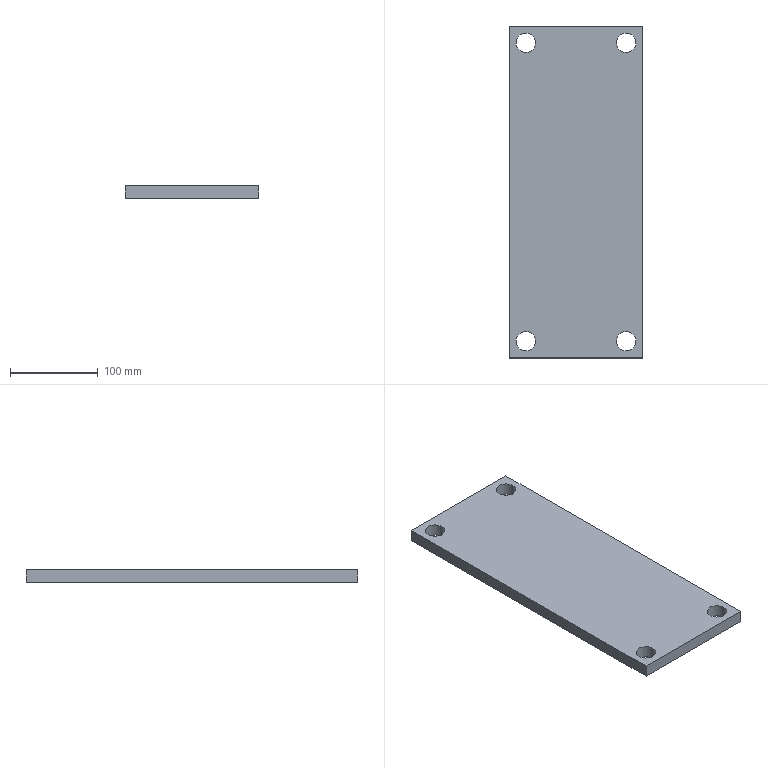Part | SolidWorks | features Extrusion 1 | 1 solid | 14 faces | box 152.4 x 377.95 x 14 mm | volume 784620 mm3 | cylinder 8 | plane 6 | commonest cylinder face diameters 22.25 x8
STEP:
#1=CARTESIAN_POINT('',(-68.275,-169.862,14.));
#2=VERTEX_POINT('',#1);
#3=CARTESIAN_POINT('',(-46.025,-169.862,14.));
#4=VERTEX_POINT('',#3);
#5=CARTESIAN_POINT('',(-57.15,-169.862,14.));
#6=DIRECTION('',(0.,0.,1.));
#7=DIRECTION('',(1.,0.,0.));
#8=AXIS2_PLACEMENT_3D('',#5,#6,#7);
#9=CIRCLE('',#8,11.125);
#10=EDGE_CURVE('',#2,#4,#9,.T.);
#11=ORIENTED_EDGE('',*,*,#10,.T.);
#12=CARTESIAN_POINT('',(-46.025,-169.862,0.));
#13=VERTEX_POINT('',#12);
#14=CARTESIAN_POINT('',(-46.025,-169.862,14.));
#15=DIRECTION('',(0.,0.,-1.));
#16=VECTOR('',#15,1000.);
#17=LINE('',#14,#16);
#18=EDGE_CURVE('',#4,#13,#17,.T.);
#19=ORIENTED_EDGE('',*,*,#18,.T.);
#20=CARTESIAN_POINT('',(-68.275,-169.862,0.));
#21=VERTEX_POINT('',#20);
#22=CARTESIAN_POINT('',(-57.15,-169.862,0.));
#23=DIRECTION('',(0.,0.,1.));
#24=DIRECTION('',(1.,0.,0.));
#25=AXIS2_PLACEMENT_3D('',#22,#23,#24);
#26=CIRCLE('',#25,11.125);
#27=EDGE_CURVE('',#21,#13,#26,.T.);
#28=ORIENTED_EDGE('',*,*,#27,.F.);
#29=CARTESIAN_POINT('',(-68.275,-169.862,14.));
#30=DIRECTION('',(0.,0.,-1.));
#31=VECTOR('',#30,1000.);
#32=LINE('',#29,#31);
#33=EDGE_CURVE('',#2,#21,#32,.T.);
#34=ORIENTED_EDGE('',*,*,#33,.F.);
#35=EDGE_LOOP('',(#11,#19,#28,#34));
#36=FACE_OUTER_BOUND('',#35,.T.);
#37=CARTESIAN_POINT('',(-57.15,-169.862,14.));
#38=DIRECTION('',(0.,0.,-1.));
#39=DIRECTION('',(-1.,0.,0.));
#40=AXIS2_PLACEMENT_3D('',#37,#38,#39);
#41=CYLINDRICAL_SURFACE('',#40,11.125);
#42=ADVANCED_FACE('',(#36),#41,.F.);
#43=CARTESIAN_POINT('',(46.025,-169.862,14.));
#44=VERTEX_POINT('',#43);
#45=CARTESIAN_POINT('',(68.275,-169.862,14.));
#46=VERTEX_POINT('',#45);
#47=CARTESIAN_POINT('',(57.15,-169.862,14.));
#48=DIRECTION('',(0.,0.,1.));
#49=DIRECTION('',(1.,0.,0.));
#50=AXIS2_PLACEMENT_3D('',#47,#48,#49);
#51=CIRCLE('',#50,11.125);
#52=EDGE_CURVE('',#44,#46,#51,.T.);
#53=ORIENTED_EDGE('',*,*,#52,.T.);
#54=CARTESIAN_POINT('',(68.275,-169.862,0.));
#55=VERTEX_POINT('',#54);
#56=CARTESIAN_POINT('',(68.275,-169.862,14.));
#57=DIRECTION('',(0.,0.,-1.));
#58=VECTOR('',#57,1000.);
#59=LINE('',#56,#58);
#60=EDGE_CURVE('',#46,#55,#59,.T.);
#61=ORIENTED_EDGE('',*,*,#60,.T.);
#62=CARTESIAN_POINT('',(46.025,-169.862,0.));
#63=VERTEX_POINT('',#62);
#64=CARTESIAN_POINT('',(57.15,-169.862,0.));
#65=DIRECTION('',(0.,0.,1.));
#66=DIRECTION('',(1.,0.,0.));
#67=AXIS2_PLACEMENT_3D('',#64,#65,#66);
#68=CIRCLE('',#67,11.125);
#69=EDGE_CURVE('',#63,#55,#68,.T.);
#70=ORIENTED_EDGE('',*,*,#69,.F.);
#71=CARTESIAN_POINT('',(46.025,-169.862,14.));
#72=DIRECTION('',(0.,0.,-1.));
#73=VECTOR('',#72,1000.);
#74=LINE('',#71,#73);
#75=EDGE_CURVE('',#44,#63,#74,.T.);
#76=ORIENTED_EDGE('',*,*,#75,.F.);
#77=EDGE_LOOP('',(#53,#61,#70,#76));
#78=FACE_OUTER_BOUND('',#77,.T.);
#79=CARTESIAN_POINT('',(57.15,-169.862,14.));
#80=DIRECTION('',(0.,0.,-1.));
#81=DIRECTION('',(-1.,0.,0.));
#82=AXIS2_PLACEMENT_3D('',#79,#80,#81);
#83=CYLINDRICAL_SURFACE('',#82,11.125);
#84=ADVANCED_FACE('',(#78),#83,.F.);
#85=CARTESIAN_POINT('',(46.025,169.863,14.));
#86=VERTEX_POINT('',#85);
#87=CARTESIAN_POINT('',(68.275,169.863,14.));
#88=VERTEX_POINT('',#87);
#89=CARTESIAN_POINT('',(57.15,169.863,14.));
#90=DIRECTION('',(0.,0.,1.));
#91=DIRECTION('',(1.,0.,0.));
#92=AXIS2_PLACEMENT_3D('',#89,#90,#91);
#93=CIRCLE('',#92,11.125);
#94=EDGE_CURVE('',#86,#88,#93,.T.);
#95=ORIENTED_EDGE('',*,*,#94,.T.);
#96=CARTESIAN_POINT('',(68.275,169.863,0.));
#97=VERTEX_POINT('',#96);
#98=CARTESIAN_POINT('',(68.275,169.863,14.));
#99=DIRECTION('',(0.,0.,-1.));
#100=VECTOR('',#99,1000.);
#101=LINE('',#98,#100);
#102=EDGE_CURVE('',#88,#97,#101,.T.);
#103=ORIENTED_EDGE('',*,*,#102,.T.);
#104=CARTESIAN_POINT('',(46.025,169.863,0.));
#105=VERTEX_POINT('',#104);
#106=CARTESIAN_POINT('',(57.15,169.863,0.));
#107=DIRECTION('',(0.,0.,1.));
#108=DIRECTION('',(1.,0.,0.));
#109=AXIS2_PLACEMENT_3D('',#106,#107,#108);
#110=CIRCLE('',#109,11.125);
#111=EDGE_CURVE('',#105,#97,#110,.T.);
#112=ORIENTED_EDGE('',*,*,#111,.F.);
#113=CARTESIAN_POINT('',(46.025,169.863,14.));
#114=DIRECTION('',(0.,0.,-1.));
#115=VECTOR('',#114,1000.);
#116=LINE('',#113,#115);
#117=EDGE_CURVE('',#86,#105,#116,.T.);
#118=ORIENTED_EDGE('',*,*,#117,.F.);
#119=EDGE_LOOP('',(#95,#103,#112,#118));
#120=FACE_OUTER_BOUND('',#119,.T.);
#121=CARTESIAN_POINT('',(57.15,169.863,14.));
#122=DIRECTION('',(0.,0.,-1.));
#123=DIRECTION('',(-1.,0.,0.));
#124=AXIS2_PLACEMENT_3D('',#121,#122,#123);
#125=CYLINDRICAL_SURFACE('',#124,11.125);
#126=ADVANCED_FACE('',(#120),#125,.F.);
#127=CARTESIAN_POINT('',(-68.275,169.863,14.));
#128=VERTEX_POINT('',#127);
#129=CARTESIAN_POINT('',(-46.025,169.863,14.));
#130=VERTEX_POINT('',#129);
#131=CARTESIAN_POINT('',(-57.15,169.863,14.));
#132=DIRECTION('',(0.,0.,1.));
#133=DIRECTION('',(1.,0.,0.));
#134=AXIS2_PLACEMENT_3D('',#131,#132,#133);
#135=CIRCLE('',#134,11.125);
#136=EDGE_CURVE('',#128,#130,#135,.T.);
#137=ORIENTED_EDGE('',*,*,#136,.T.);
#138=CARTESIAN_POINT('',(-46.025,169.863,0.));
#139=VERTEX_POINT('',#138);
#140=CARTESIAN_POINT('',(-46.025,169.863,14.));
#141=DIRECTION('',(0.,0.,-1.));
#142=VECTOR('',#141,1000.);
#143=LINE('',#140,#142);
#144=EDGE_CURVE('',#130,#139,#143,.T.);
#145=ORIENTED_EDGE('',*,*,#144,.T.);
#146=CARTESIAN_POINT('',(-68.275,169.863,0.));
#147=VERTEX_POINT('',#146);
#148=CARTESIAN_POINT('',(-57.15,169.863,0.));
#149=DIRECTION('',(0.,0.,1.));
#150=DIRECTION('',(1.,0.,0.));
#151=AXIS2_PLACEMENT_3D('',#148,#149,#150);
#152=CIRCLE('',#151,11.125);
#153=EDGE_CURVE('',#147,#139,#152,.T.);
#154=ORIENTED_EDGE('',*,*,#153,.F.);
#155=CARTESIAN_POINT('',(-68.275,169.863,14.));
#156=DIRECTION('',(0.,0.,-1.));
#157=VECTOR('',#156,1000.);
#158=LINE('',#155,#157);
#159=EDGE_CURVE('',#128,#147,#158,.T.);
#160=ORIENTED_EDGE('',*,*,#159,.F.);
#161=EDGE_LOOP('',(#137,#145,#154,#160));
#162=FACE_OUTER_BOUND('',#161,.T.);
#163=CARTESIAN_POINT('',(-57.15,169.863,14.));
#164=DIRECTION('',(0.,0.,-1.));
#165=DIRECTION('',(-1.,0.,0.));
#166=AXIS2_PLACEMENT_3D('',#163,#164,#165);
#167=CYLINDRICAL_SURFACE('',#166,11.125);
#168=ADVANCED_FACE('',(#162),#167,.F.);
#169=ORIENTED_EDGE('',*,*,#52,.F.);
#170=CARTESIAN_POINT('',(57.15,-169.862,14.));
#171=DIRECTION('',(0.,0.,1.));
#172=DIRECTION('',(1.,0.,0.));
#173=AXIS2_PLACEMENT_3D('',#170,#171,#172);
#174=CIRCLE('',#173,11.125);
#175=EDGE_CURVE('',#46,#44,#174,.T.);
#176=ORIENTED_EDGE('',*,*,#175,.F.);
#177=EDGE_LOOP('',(#169,#176));
#178=FACE_BOUND('',#177,.T.);
#179=ORIENTED_EDGE('',*,*,#136,.F.);
#180=CARTESIAN_POINT('',(-57.15,169.863,14.));
#181=DIRECTION('',(0.,0.,1.));
#182=DIRECTION('',(1.,0.,0.));
#183=AXIS2_PLACEMENT_3D('',#180,#181,#182);
#184=CIRCLE('',#183,11.125);
#185=EDGE_CURVE('',#130,#128,#184,.T.);
#186=ORIENTED_EDGE('',*,*,#185,.F.);
#187=EDGE_LOOP('',(#179,#186));
#188=FACE_BOUND('',#187,.T.);
#189=CARTESIAN_POINT('',(76.2,-188.975,14.));
#190=VERTEX_POINT('',#189);
#191=CARTESIAN_POINT('',(76.2,188.975,14.));
#192=VERTEX_POINT('',#191);
#193=CARTESIAN_POINT('',(76.2,188.975,14.));
#194=DIRECTION('',(0.,1.,0.));
#195=VECTOR('',#194,1000.);
#196=LINE('',#193,#195);
#197=EDGE_CURVE('',#190,#192,#196,.T.);
#198=ORIENTED_EDGE('',*,*,#197,.T.);
#199=CARTESIAN_POINT('',(-76.2,188.975,14.));
#200=VERTEX_POINT('',#199);
#201=CARTESIAN_POINT('',(-76.2,188.975,14.));
#202=DIRECTION('',(-1.,0.,0.));
#203=VECTOR('',#202,1000.);
#204=LINE('',#201,#203);
#205=EDGE_CURVE('',#192,#200,#204,.T.);
#206=ORIENTED_EDGE('',*,*,#205,.T.);
#207=CARTESIAN_POINT('',(-76.2,-188.975,14.));
#208=VERTEX_POINT('',#207);
#209=CARTESIAN_POINT('',(-76.2,188.975,14.));
#210=DIRECTION('',(0.,-1.,0.));
#211=VECTOR('',#210,1000.);
#212=LINE('',#209,#211);
#213=EDGE_CURVE('',#200,#208,#212,.T.);
#214=ORIENTED_EDGE('',*,*,#213,.T.);
#215=CARTESIAN_POINT('',(-76.2,-188.975,14.));
#216=DIRECTION('',(1.,0.,0.));
#217=VECTOR('',#216,1000.);
#218=LINE('',#215,#217);
#219=EDGE_CURVE('',#208,#190,#218,.T.);
#220=ORIENTED_EDGE('',*,*,#219,.T.);
#221=EDGE_LOOP('',(#198,#206,#214,#220));
#222=FACE_OUTER_BOUND('',#221,.T.);
#223=ORIENTED_EDGE('',*,*,#94,.F.);
#224=CARTESIAN_POINT('',(57.15,169.863,14.));
#225=DIRECTION('',(0.,0.,1.));
#226=DIRECTION('',(1.,0.,0.));
#227=AXIS2_PLACEMENT_3D('',#224,#225,#226);
#228=CIRCLE('',#227,11.125);
#229=EDGE_CURVE('',#88,#86,#228,.T.);
#230=ORIENTED_EDGE('',*,*,#229,.F.);
#231=EDGE_LOOP('',(#223,#230));
#232=FACE_BOUND('',#231,.T.);
#233=ORIENTED_EDGE('',*,*,#10,.F.);
#234=CARTESIAN_POINT('',(-57.15,-169.862,14.));
#235=DIRECTION('',(0.,0.,1.));
#236=DIRECTION('',(1.,0.,0.));
#237=AXIS2_PLACEMENT_3D('',#234,#235,#236);
#238=CIRCLE('',#237,11.125);
#239=EDGE_CURVE('',#4,#2,#238,.T.);
#240=ORIENTED_EDGE('',*,*,#239,.F.);
#241=EDGE_LOOP('',(#233,#240));
#242=FACE_BOUND('',#241,.T.);
#243=CARTESIAN_POINT('',(76.2,-188.975,14.));
#244=DIRECTION('',(0.,0.,1.));
#245=DIRECTION('',(1.,0.,0.));
#246=AXIS2_PLACEMENT_3D('',#243,#244,#245);
#247=PLANE('',#246);
#248=ADVANCED_FACE('',(#178,#188,#222,#232,#242),#247,.T.);
#249=ORIENTED_EDGE('',*,*,#69,.T.);
#250=CARTESIAN_POINT('',(57.15,-169.862,0.));
#251=DIRECTION('',(0.,0.,1.));
#252=DIRECTION('',(1.,0.,0.));
#253=AXIS2_PLACEMENT_3D('',#250,#251,#252);
#254=CIRCLE('',#253,11.125);
#255=EDGE_CURVE('',#55,#63,#254,.T.);
#256=ORIENTED_EDGE('',*,*,#255,.T.);
#257=EDGE_LOOP('',(#249,#256));
#258=FACE_BOUND('',#257,.T.);
#259=ORIENTED_EDGE('',*,*,#153,.T.);
#260=CARTESIAN_POINT('',(-57.15,169.863,0.));
#261=DIRECTION('',(0.,0.,1.));
#262=DIRECTION('',(1.,0.,0.));
#263=AXIS2_PLACEMENT_3D('',#260,#261,#262);
#264=CIRCLE('',#263,11.125);
#265=EDGE_CURVE('',#139,#147,#264,.T.);
#266=ORIENTED_EDGE('',*,*,#265,.T.);
#267=EDGE_LOOP('',(#259,#266));
#268=FACE_BOUND('',#267,.T.);
#269=CARTESIAN_POINT('',(76.2,-188.975,0.));
#270=VERTEX_POINT('',#269);
#271=CARTESIAN_POINT('',(76.2,188.975,0.));
#272=VERTEX_POINT('',#271);
#273=CARTESIAN_POINT('',(76.2,188.975,0.));
#274=DIRECTION('',(0.,1.,0.));
#275=VECTOR('',#274,1000.);
#276=LINE('',#273,#275);
#277=EDGE_CURVE('',#270,#272,#276,.T.);
#278=ORIENTED_EDGE('',*,*,#277,.F.);
#279=CARTESIAN_POINT('',(-76.2,-188.975,0.));
#280=VERTEX_POINT('',#279);
#281=CARTESIAN_POINT('',(-76.2,-188.975,0.));
#282=DIRECTION('',(1.,0.,0.));
#283=VECTOR('',#282,1000.);
#284=LINE('',#281,#283);
#285=EDGE_CURVE('',#280,#270,#284,.T.);
#286=ORIENTED_EDGE('',*,*,#285,.F.);
#287=CARTESIAN_POINT('',(-76.2,188.975,0.));
#288=VERTEX_POINT('',#287);
#289=CARTESIAN_POINT('',(-76.2,188.975,0.));
#290=DIRECTION('',(0.,-1.,0.));
#291=VECTOR('',#290,1000.);
#292=LINE('',#289,#291);
#293=EDGE_CURVE('',#288,#280,#292,.T.);
#294=ORIENTED_EDGE('',*,*,#293,.F.);
#295=CARTESIAN_POINT('',(-76.2,188.975,0.));
#296=DIRECTION('',(-1.,0.,0.));
#297=VECTOR('',#296,1000.);
#298=LINE('',#295,#297);
#299=EDGE_CURVE('',#272,#288,#298,.T.);
#300=ORIENTED_EDGE('',*,*,#299,.F.);
#301=EDGE_LOOP('',(#278,#286,#294,#300));
#302=FACE_OUTER_BOUND('',#301,.T.);
#303=ORIENTED_EDGE('',*,*,#111,.T.);
#304=CARTESIAN_POINT('',(57.15,169.863,0.));
#305=DIRECTION('',(0.,0.,1.));
#306=DIRECTION('',(1.,0.,0.));
#307=AXIS2_PLACEMENT_3D('',#304,#305,#306);
#308=CIRCLE('',#307,11.125);
#309=EDGE_CURVE('',#97,#105,#308,.T.);
#310=ORIENTED_EDGE('',*,*,#309,.T.);
#311=EDGE_LOOP('',(#303,#310));
#312=FACE_BOUND('',#311,.T.);
#313=ORIENTED_EDGE('',*,*,#27,.T.);
#314=CARTESIAN_POINT('',(-57.15,-169.862,0.));
#315=DIRECTION('',(0.,0.,1.));
#316=DIRECTION('',(1.,0.,0.));
#317=AXIS2_PLACEMENT_3D('',#314,#315,#316);
#318=CIRCLE('',#317,11.125);
#319=EDGE_CURVE('',#13,#21,#318,.T.);
#320=ORIENTED_EDGE('',*,*,#319,.T.);
#321=EDGE_LOOP('',(#313,#320));
#322=FACE_BOUND('',#321,.T.);
#323=CARTESIAN_POINT('',(76.2,-188.975,0.));
#324=DIRECTION('',(0.,0.,1.));
#325=DIRECTION('',(1.,0.,0.));
#326=AXIS2_PLACEMENT_3D('',#323,#324,#325);
#327=PLANE('',#326);
#328=ADVANCED_FACE('',(#258,#268,#302,#312,#322),#327,.F.);
#329=ORIENTED_EDGE('',*,*,#277,.T.);
#330=CARTESIAN_POINT('',(76.2,188.975,14.));
#331=DIRECTION('',(0.,0.,-1.));
#332=VECTOR('',#331,1000.);
#333=LINE('',#330,#332);
#334=EDGE_CURVE('',#192,#272,#333,.T.);
#335=ORIENTED_EDGE('',*,*,#334,.F.);
#336=ORIENTED_EDGE('',*,*,#197,.F.);
#337=CARTESIAN_POINT('',(76.2,-188.975,14.));
#338=DIRECTION('',(0.,0.,-1.));
#339=VECTOR('',#338,1000.);
#340=LINE('',#337,#339);
#341=EDGE_CURVE('',#190,#270,#340,.T.);
#342=ORIENTED_EDGE('',*,*,#341,.T.);
#343=EDGE_LOOP('',(#329,#335,#336,#342));
#344=FACE_OUTER_BOUND('',#343,.T.);
#345=CARTESIAN_POINT('',(76.2,188.975,14.));
#346=DIRECTION('',(-1.,0.,0.));
#347=DIRECTION('',(0.,-1.,0.));
#348=AXIS2_PLACEMENT_3D('',#345,#346,#347);
#349=PLANE('',#348);
#350=ADVANCED_FACE('',(#344),#349,.F.);
#351=ORIENTED_EDGE('',*,*,#299,.T.);
#352=CARTESIAN_POINT('',(-76.2,188.975,14.));
#353=DIRECTION('',(0.,0.,-1.));
#354=VECTOR('',#353,1000.);
#355=LINE('',#352,#354);
#356=EDGE_CURVE('',#200,#288,#355,.T.);
#357=ORIENTED_EDGE('',*,*,#356,.F.);
#358=ORIENTED_EDGE('',*,*,#205,.F.);
#359=ORIENTED_EDGE('',*,*,#334,.T.);
#360=EDGE_LOOP('',(#351,#357,#358,#359));
#361=FACE_OUTER_BOUND('',#360,.T.);
#362=CARTESIAN_POINT('',(-76.2,188.975,14.));
#363=DIRECTION('',(0.,-1.,0.));
#364=DIRECTION('',(0.,0.,-1.));
#365=AXIS2_PLACEMENT_3D('',#362,#363,#364);
#366=PLANE('',#365);
#367=ADVANCED_FACE('',(#361),#366,.F.);
#368=ORIENTED_EDGE('',*,*,#293,.T.);
#369=CARTESIAN_POINT('',(-76.2,-188.975,14.));
#370=DIRECTION('',(0.,0.,-1.));
#371=VECTOR('',#370,1000.);
#372=LINE('',#369,#371);
#373=EDGE_CURVE('',#208,#280,#372,.T.);
#374=ORIENTED_EDGE('',*,*,#373,.F.);
#375=ORIENTED_EDGE('',*,*,#213,.F.);
#376=ORIENTED_EDGE('',*,*,#356,.T.);
#377=EDGE_LOOP('',(#368,#374,#375,#376));
#378=FACE_OUTER_BOUND('',#377,.T.);
#379=CARTESIAN_POINT('',(-76.2,188.975,14.));
#380=DIRECTION('',(1.,0.,0.));
#381=DIRECTION('',(0.,1.,0.));
#382=AXIS2_PLACEMENT_3D('',#379,#380,#381);
#383=PLANE('',#382);
#384=ADVANCED_FACE('',(#378),#383,.F.);
#385=ORIENTED_EDGE('',*,*,#285,.T.);
#386=ORIENTED_EDGE('',*,*,#341,.F.);
#387=ORIENTED_EDGE('',*,*,#219,.F.);
#388=ORIENTED_EDGE('',*,*,#373,.T.);
#389=EDGE_LOOP('',(#385,#386,#387,#388));
#390=FACE_OUTER_BOUND('',#389,.T.);
#391=CARTESIAN_POINT('',(-76.2,-188.975,14.));
#392=DIRECTION('',(0.,1.,0.));
#393=DIRECTION('',(0.,0.,1.));
#394=AXIS2_PLACEMENT_3D('',#391,#392,#393);
#395=PLANE('',#394);
#396=ADVANCED_FACE('',(#390),#395,.F.);
#397=ORIENTED_EDGE('',*,*,#144,.F.);
#398=ORIENTED_EDGE('',*,*,#185,.T.);
#399=ORIENTED_EDGE('',*,*,#159,.T.);
#400=ORIENTED_EDGE('',*,*,#265,.F.);
#401=EDGE_LOOP('',(#397,#398,#399,#400));
#402=FACE_OUTER_BOUND('',#401,.T.);
#403=CARTESIAN_POINT('',(-57.15,169.863,14.));
#404=DIRECTION('',(0.,0.,-1.));
#405=DIRECTION('',(-1.,0.,0.));
#406=AXIS2_PLACEMENT_3D('',#403,#404,#405);
#407=CYLINDRICAL_SURFACE('',#406,11.125);
#408=ADVANCED_FACE('',(#402),#407,.F.);
#409=ORIENTED_EDGE('',*,*,#102,.F.);
#410=ORIENTED_EDGE('',*,*,#229,.T.);
#411=ORIENTED_EDGE('',*,*,#117,.T.);
#412=ORIENTED_EDGE('',*,*,#309,.F.);
#413=EDGE_LOOP('',(#409,#410,#411,#412));
#414=FACE_OUTER_BOUND('',#413,.T.);
#415=CARTESIAN_POINT('',(57.15,169.863,14.));
#416=DIRECTION('',(0.,0.,-1.));
#417=DIRECTION('',(-1.,0.,0.));
#418=AXIS2_PLACEMENT_3D('',#415,#416,#417);
#419=CYLINDRICAL_SURFACE('',#418,11.125);
#420=ADVANCED_FACE('',(#414),#419,.F.);
#421=ORIENTED_EDGE('',*,*,#60,.F.);
#422=ORIENTED_EDGE('',*,*,#175,.T.);
#423=ORIENTED_EDGE('',*,*,#75,.T.);
#424=ORIENTED_EDGE('',*,*,#255,.F.);
#425=EDGE_LOOP('',(#421,#422,#423,#424));
#426=FACE_OUTER_BOUND('',#425,.T.);
#427=CARTESIAN_POINT('',(57.15,-169.862,14.));
#428=DIRECTION('',(0.,0.,-1.));
#429=DIRECTION('',(-1.,0.,0.));
#430=AXIS2_PLACEMENT_3D('',#427,#428,#429);
#431=CYLINDRICAL_SURFACE('',#430,11.125);
#432=ADVANCED_FACE('',(#426),#431,.F.);
#433=ORIENTED_EDGE('',*,*,#18,.F.);
#434=ORIENTED_EDGE('',*,*,#239,.T.);
#435=ORIENTED_EDGE('',*,*,#33,.T.);
#436=ORIENTED_EDGE('',*,*,#319,.F.);
#437=EDGE_LOOP('',(#433,#434,#435,#436));
#438=FACE_OUTER_BOUND('',#437,.T.);
#439=CARTESIAN_POINT('',(-57.15,-169.862,14.));
#440=DIRECTION('',(0.,0.,-1.));
#441=DIRECTION('',(-1.,0.,0.));
#442=AXIS2_PLACEMENT_3D('',#439,#440,#441);
#443=CYLINDRICAL_SURFACE('',#442,11.125);
#444=ADVANCED_FACE('',(#438),#443,.F.);
#445=CLOSED_SHELL('',(#42,#84,#126,#168,#248,#328,#350,#367,#384,#396,#408,#420,#432,#444));
#446=MANIFOLD_SOLID_BREP('',#445);
#447=CARTESIAN_POINT('',(0.,0.,0.));
#448=DIRECTION('',(0.,0.,1.));
#449=DIRECTION('',(1.,0.,0.));
#450=AXIS2_PLACEMENT_3D('',#447,#448,#449);
#451=(LENGTH_UNIT()NAMED_UNIT(*)SI_UNIT(.MILLI.,.METRE.));
#452=UNCERTAINTY_MEASURE_WITH_UNIT(LENGTH_MEASURE(0.00001),#451,'','');
#453=(NAMED_UNIT(*)PLANE_ANGLE_UNIT()SI_UNIT($,.RADIAN.));
#454=(NAMED_UNIT(*)SI_UNIT($,.STERADIAN.)SOLID_ANGLE_UNIT());
#455=(GEOMETRIC_REPRESENTATION_CONTEXT(3)GLOBAL_UNCERTAINTY_ASSIGNED_CONTEXT((#452))GLOBAL_UNIT_ASSIGNED_CONTEXT((#451,#453,#454))REPRESENTATION_CONTEXT('',''));
#456=ADVANCED_BREP_SHAPE_REPRESENTATION('',(#446,#450),#455);